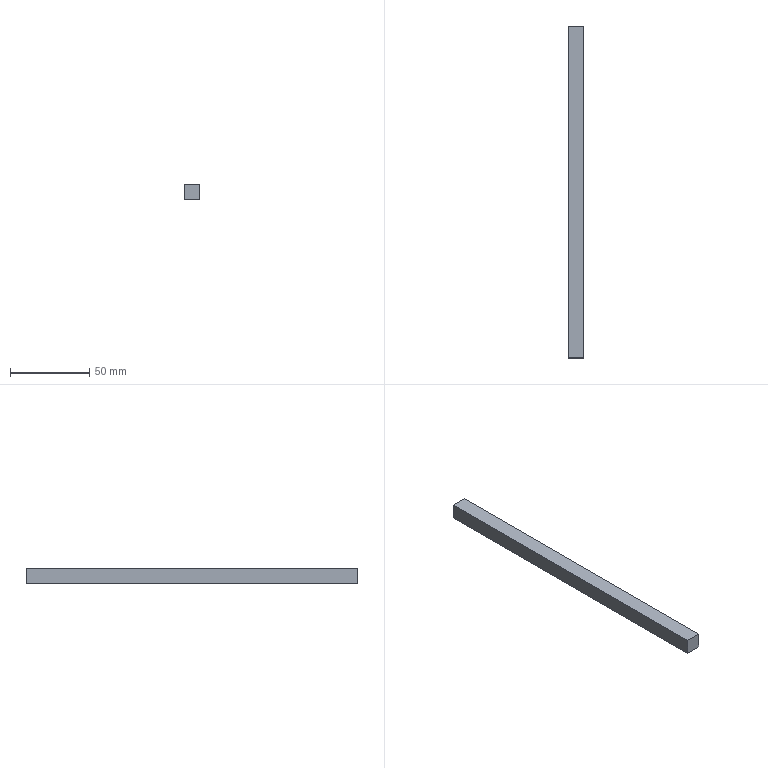Part | STEP file | 001-004-Feeding mechanism shaft entry channel baffle | 1 solid | 6 faces | box 10 x 210 x 10 mm | volume 21000 mm3 | plane 6
STEP:
#1=CARTESIAN_POINT('',(0.,0.,0.));
#2=DIRECTION('',(0.,0.,1.));
#3=DIRECTION('',(1.,0.,0.));
#4=AXIS2_PLACEMENT_3D('',#1,#2,#3);
#5=CARTESIAN_POINT('',(5.,-105.,0.));
#6=VERTEX_POINT('',#5);
#7=CARTESIAN_POINT('',(5.,105.,0.));
#8=VERTEX_POINT('',#7);
#9=CARTESIAN_POINT('',(5.,-105.,0.));
#10=DIRECTION('',(0.,1.,0.));
#11=VECTOR('',#10,1.);
#12=LINE('',#9,#11);
#13=CARTESIAN_POINT('',(5.,-105.,10.));
#14=DIRECTION('',(-1.,0.,0.));
#15=DIRECTION('',(0.,0.,1.));
#16=AXIS2_PLACEMENT_3D('',#13,#14,#15);
#17=PLANE('',#16);
#18=CARTESIAN_POINT('',(-10.,0.));
#19=DIRECTION('',(0.,1.));
#20=VECTOR('',#19,1.);
#21=LINE('',#18,#20);
#22=(GEOMETRIC_REPRESENTATION_CONTEXT(2)PARAMETRIC_REPRESENTATION_CONTEXT()REPRESENTATION_CONTEXT('',''));
#23=DEFINITIONAL_REPRESENTATION('',(#21),#22);
#24=PCURVE('',#17,#23);
#25=CARTESIAN_POINT('',(0.,0.,0.));
#26=DIRECTION('',(0.,0.,-1.));
#27=DIRECTION('',(-1.,0.,0.));
#28=AXIS2_PLACEMENT_3D('',#25,#26,#27);
#29=PLANE('',#28);
#30=CARTESIAN_POINT('',(-5.,-105.));
#31=DIRECTION('',(0.,1.));
#32=VECTOR('',#31,1.);
#33=LINE('',#30,#32);
#34=(GEOMETRIC_REPRESENTATION_CONTEXT(2)PARAMETRIC_REPRESENTATION_CONTEXT()REPRESENTATION_CONTEXT('',''));
#35=DEFINITIONAL_REPRESENTATION('',(#33),#34);
#36=PCURVE('',#29,#35);
#37=SURFACE_CURVE('',#12,(#24,#36),.PCURVE_S1.);
#38=EDGE_CURVE('',#6,#8,#37,.T.);
#39=ORIENTED_EDGE('',*,*,#38,.T.);
#40=CARTESIAN_POINT('',(5.,105.,10.));
#41=VERTEX_POINT('',#40);
#42=CARTESIAN_POINT('',(5.,105.,10.));
#43=DIRECTION('',(0.,0.,-1.));
#44=VECTOR('',#43,1.);
#45=LINE('',#42,#44);
#46=CARTESIAN_POINT('',(0.,210.));
#47=DIRECTION('',(-1.,0.));
#48=VECTOR('',#47,1.);
#49=LINE('',#46,#48);
#50=(GEOMETRIC_REPRESENTATION_CONTEXT(2)PARAMETRIC_REPRESENTATION_CONTEXT()REPRESENTATION_CONTEXT('',''));
#51=DEFINITIONAL_REPRESENTATION('',(#49),#50);
#52=PCURVE('',#17,#51);
#53=CARTESIAN_POINT('',(-5.,105.,10.));
#54=DIRECTION('',(0.,-1.,0.));
#55=DIRECTION('',(0.,0.,-1.));
#56=AXIS2_PLACEMENT_3D('',#53,#54,#55);
#57=PLANE('',#56);
#58=CARTESIAN_POINT('',(0.,10.));
#59=DIRECTION('',(1.,0.));
#60=VECTOR('',#59,1.);
#61=LINE('',#58,#60);
#62=(GEOMETRIC_REPRESENTATION_CONTEXT(2)PARAMETRIC_REPRESENTATION_CONTEXT()REPRESENTATION_CONTEXT('',''));
#63=DEFINITIONAL_REPRESENTATION('',(#61),#62);
#64=PCURVE('',#57,#63);
#65=SURFACE_CURVE('',#45,(#52,#64),.PCURVE_S1.);
#66=EDGE_CURVE('',#41,#8,#65,.T.);
#67=ORIENTED_EDGE('',*,*,#66,.F.);
#68=CARTESIAN_POINT('',(5.,-105.,10.));
#69=VERTEX_POINT('',#68);
#70=CARTESIAN_POINT('',(5.,-105.,10.));
#71=DIRECTION('',(0.,1.,0.));
#72=VECTOR('',#71,1.);
#73=LINE('',#70,#72);
#74=CARTESIAN_POINT('',(0.,0.));
#75=DIRECTION('',(0.,1.));
#76=VECTOR('',#75,1.);
#77=LINE('',#74,#76);
#78=(GEOMETRIC_REPRESENTATION_CONTEXT(2)PARAMETRIC_REPRESENTATION_CONTEXT()REPRESENTATION_CONTEXT('',''));
#79=DEFINITIONAL_REPRESENTATION('',(#77),#78);
#80=PCURVE('',#17,#79);
#81=CARTESIAN_POINT('',(0.,0.,10.));
#82=DIRECTION('',(0.,0.,-1.));
#83=DIRECTION('',(-1.,0.,0.));
#84=AXIS2_PLACEMENT_3D('',#81,#82,#83);
#85=PLANE('',#84);
#86=CARTESIAN_POINT('',(-5.,-105.));
#87=DIRECTION('',(0.,1.));
#88=VECTOR('',#87,1.);
#89=LINE('',#86,#88);
#90=(GEOMETRIC_REPRESENTATION_CONTEXT(2)PARAMETRIC_REPRESENTATION_CONTEXT()REPRESENTATION_CONTEXT('',''));
#91=DEFINITIONAL_REPRESENTATION('',(#89),#90);
#92=PCURVE('',#85,#91);
#93=SURFACE_CURVE('',#73,(#80,#92),.PCURVE_S1.);
#94=EDGE_CURVE('',#69,#41,#93,.T.);
#95=ORIENTED_EDGE('',*,*,#94,.F.);
#96=CARTESIAN_POINT('',(5.,-105.,10.));
#97=DIRECTION('',(0.,0.,-1.));
#98=VECTOR('',#97,1.);
#99=LINE('',#96,#98);
#100=CARTESIAN_POINT('',(0.,0.));
#101=DIRECTION('',(-1.,0.));
#102=VECTOR('',#101,1.);
#103=LINE('',#100,#102);
#104=(GEOMETRIC_REPRESENTATION_CONTEXT(2)PARAMETRIC_REPRESENTATION_CONTEXT()REPRESENTATION_CONTEXT('',''));
#105=DEFINITIONAL_REPRESENTATION('',(#103),#104);
#106=PCURVE('',#17,#105);
#107=CARTESIAN_POINT('',(-5.,-105.,10.));
#108=DIRECTION('',(0.,1.,0.));
#109=DIRECTION('',(0.,0.,1.));
#110=AXIS2_PLACEMENT_3D('',#107,#108,#109);
#111=PLANE('',#110);
#112=CARTESIAN_POINT('',(0.,10.));
#113=DIRECTION('',(-1.,0.));
#114=VECTOR('',#113,1.);
#115=LINE('',#112,#114);
#116=(GEOMETRIC_REPRESENTATION_CONTEXT(2)PARAMETRIC_REPRESENTATION_CONTEXT()REPRESENTATION_CONTEXT('',''));
#117=DEFINITIONAL_REPRESENTATION('',(#115),#116);
#118=PCURVE('',#111,#117);
#119=SURFACE_CURVE('',#99,(#106,#118),.PCURVE_S1.);
#120=EDGE_CURVE('',#69,#6,#119,.T.);
#121=ORIENTED_EDGE('',*,*,#120,.T.);
#122=EDGE_LOOP('',(#39,#67,#95,#121));
#123=FACE_BOUND('',#122,.T.);
#124=ADVANCED_FACE('',(#123),#17,.F.);
#125=CARTESIAN_POINT('',(-5.,105.,0.));
#126=VERTEX_POINT('',#125);
#127=CARTESIAN_POINT('',(-5.,105.,0.));
#128=DIRECTION('',(-1.,0.,0.));
#129=VECTOR('',#128,1.);
#130=LINE('',#127,#129);
#131=CARTESIAN_POINT('',(10.,0.));
#132=DIRECTION('',(0.,-1.));
#133=VECTOR('',#132,1.);
#134=LINE('',#131,#133);
#135=(GEOMETRIC_REPRESENTATION_CONTEXT(2)PARAMETRIC_REPRESENTATION_CONTEXT()REPRESENTATION_CONTEXT('',''));
#136=DEFINITIONAL_REPRESENTATION('',(#134),#135);
#137=PCURVE('',#57,#136);
#138=CARTESIAN_POINT('',(5.,105.));
#139=DIRECTION('',(1.,0.));
#140=VECTOR('',#139,1.);
#141=LINE('',#138,#140);
#142=(GEOMETRIC_REPRESENTATION_CONTEXT(2)PARAMETRIC_REPRESENTATION_CONTEXT()REPRESENTATION_CONTEXT('',''));
#143=DEFINITIONAL_REPRESENTATION('',(#141),#142);
#144=PCURVE('',#29,#143);
#145=SURFACE_CURVE('',#130,(#137,#144),.PCURVE_S1.);
#146=EDGE_CURVE('',#8,#126,#145,.T.);
#147=ORIENTED_EDGE('',*,*,#146,.T.);
#148=CARTESIAN_POINT('',(-5.,105.,10.));
#149=VERTEX_POINT('',#148);
#150=CARTESIAN_POINT('',(-5.,105.,10.));
#151=DIRECTION('',(0.,0.,-1.));
#152=VECTOR('',#151,1.);
#153=LINE('',#150,#152);
#154=CARTESIAN_POINT('',(0.,0.));
#155=DIRECTION('',(1.,0.));
#156=VECTOR('',#155,1.);
#157=LINE('',#154,#156);
#158=(GEOMETRIC_REPRESENTATION_CONTEXT(2)PARAMETRIC_REPRESENTATION_CONTEXT()REPRESENTATION_CONTEXT('',''));
#159=DEFINITIONAL_REPRESENTATION('',(#157),#158);
#160=PCURVE('',#57,#159);
#161=CARTESIAN_POINT('',(-5.,-105.,10.));
#162=DIRECTION('',(1.,0.,0.));
#163=DIRECTION('',(0.,0.,-1.));
#164=AXIS2_PLACEMENT_3D('',#161,#162,#163);
#165=PLANE('',#164);
#166=CARTESIAN_POINT('',(0.,210.));
#167=DIRECTION('',(1.,0.));
#168=VECTOR('',#167,1.);
#169=LINE('',#166,#168);
#170=(GEOMETRIC_REPRESENTATION_CONTEXT(2)PARAMETRIC_REPRESENTATION_CONTEXT()REPRESENTATION_CONTEXT('',''));
#171=DEFINITIONAL_REPRESENTATION('',(#169),#170);
#172=PCURVE('',#165,#171);
#173=SURFACE_CURVE('',#153,(#160,#172),.PCURVE_S1.);
#174=EDGE_CURVE('',#149,#126,#173,.T.);
#175=ORIENTED_EDGE('',*,*,#174,.F.);
#176=CARTESIAN_POINT('',(-5.,105.,10.));
#177=DIRECTION('',(-1.,0.,0.));
#178=VECTOR('',#177,1.);
#179=LINE('',#176,#178);
#180=CARTESIAN_POINT('',(0.,0.));
#181=DIRECTION('',(0.,-1.));
#182=VECTOR('',#181,1.);
#183=LINE('',#180,#182);
#184=(GEOMETRIC_REPRESENTATION_CONTEXT(2)PARAMETRIC_REPRESENTATION_CONTEXT()REPRESENTATION_CONTEXT('',''));
#185=DEFINITIONAL_REPRESENTATION('',(#183),#184);
#186=PCURVE('',#57,#185);
#187=CARTESIAN_POINT('',(5.,105.));
#188=DIRECTION('',(1.,0.));
#189=VECTOR('',#188,1.);
#190=LINE('',#187,#189);
#191=(GEOMETRIC_REPRESENTATION_CONTEXT(2)PARAMETRIC_REPRESENTATION_CONTEXT()REPRESENTATION_CONTEXT('',''));
#192=DEFINITIONAL_REPRESENTATION('',(#190),#191);
#193=PCURVE('',#85,#192);
#194=SURFACE_CURVE('',#179,(#186,#193),.PCURVE_S1.);
#195=EDGE_CURVE('',#41,#149,#194,.T.);
#196=ORIENTED_EDGE('',*,*,#195,.F.);
#197=ORIENTED_EDGE('',*,*,#66,.T.);
#198=EDGE_LOOP('',(#147,#175,#196,#197));
#199=FACE_BOUND('',#198,.T.);
#200=ADVANCED_FACE('',(#199),#57,.F.);
#201=CARTESIAN_POINT('',(-5.,-105.,0.));
#202=VERTEX_POINT('',#201);
#203=CARTESIAN_POINT('',(-5.,-105.,0.));
#204=DIRECTION('',(0.,-1.,0.));
#205=VECTOR('',#204,1.);
#206=LINE('',#203,#205);
#207=CARTESIAN_POINT('',(10.,0.));
#208=DIRECTION('',(0.,-1.));
#209=VECTOR('',#208,1.);
#210=LINE('',#207,#209);
#211=(GEOMETRIC_REPRESENTATION_CONTEXT(2)PARAMETRIC_REPRESENTATION_CONTEXT()REPRESENTATION_CONTEXT('',''));
#212=DEFINITIONAL_REPRESENTATION('',(#210),#211);
#213=PCURVE('',#165,#212);
#214=CARTESIAN_POINT('',(5.,-105.));
#215=DIRECTION('',(0.,-1.));
#216=VECTOR('',#215,1.);
#217=LINE('',#214,#216);
#218=(GEOMETRIC_REPRESENTATION_CONTEXT(2)PARAMETRIC_REPRESENTATION_CONTEXT()REPRESENTATION_CONTEXT('',''));
#219=DEFINITIONAL_REPRESENTATION('',(#217),#218);
#220=PCURVE('',#29,#219);
#221=SURFACE_CURVE('',#206,(#213,#220),.PCURVE_S1.);
#222=EDGE_CURVE('',#126,#202,#221,.T.);
#223=ORIENTED_EDGE('',*,*,#222,.T.);
#224=CARTESIAN_POINT('',(-5.,-105.,10.));
#225=VERTEX_POINT('',#224);
#226=CARTESIAN_POINT('',(-5.,-105.,10.));
#227=DIRECTION('',(0.,0.,-1.));
#228=VECTOR('',#227,1.);
#229=LINE('',#226,#228);
#230=CARTESIAN_POINT('',(0.,0.));
#231=DIRECTION('',(1.,0.));
#232=VECTOR('',#231,1.);
#233=LINE('',#230,#232);
#234=(GEOMETRIC_REPRESENTATION_CONTEXT(2)PARAMETRIC_REPRESENTATION_CONTEXT()REPRESENTATION_CONTEXT('',''));
#235=DEFINITIONAL_REPRESENTATION('',(#233),#234);
#236=PCURVE('',#165,#235);
#237=CARTESIAN_POINT('',(0.,0.));
#238=DIRECTION('',(-1.,0.));
#239=VECTOR('',#238,1.);
#240=LINE('',#237,#239);
#241=(GEOMETRIC_REPRESENTATION_CONTEXT(2)PARAMETRIC_REPRESENTATION_CONTEXT()REPRESENTATION_CONTEXT('',''));
#242=DEFINITIONAL_REPRESENTATION('',(#240),#241);
#243=PCURVE('',#111,#242);
#244=SURFACE_CURVE('',#229,(#236,#243),.PCURVE_S1.);
#245=EDGE_CURVE('',#225,#202,#244,.T.);
#246=ORIENTED_EDGE('',*,*,#245,.F.);
#247=CARTESIAN_POINT('',(-5.,-105.,10.));
#248=DIRECTION('',(0.,-1.,0.));
#249=VECTOR('',#248,1.);
#250=LINE('',#247,#249);
#251=CARTESIAN_POINT('',(0.,0.));
#252=DIRECTION('',(0.,-1.));
#253=VECTOR('',#252,1.);
#254=LINE('',#251,#253);
#255=(GEOMETRIC_REPRESENTATION_CONTEXT(2)PARAMETRIC_REPRESENTATION_CONTEXT()REPRESENTATION_CONTEXT('',''));
#256=DEFINITIONAL_REPRESENTATION('',(#254),#255);
#257=PCURVE('',#165,#256);
#258=CARTESIAN_POINT('',(5.,-105.));
#259=DIRECTION('',(0.,-1.));
#260=VECTOR('',#259,1.);
#261=LINE('',#258,#260);
#262=(GEOMETRIC_REPRESENTATION_CONTEXT(2)PARAMETRIC_REPRESENTATION_CONTEXT()REPRESENTATION_CONTEXT('',''));
#263=DEFINITIONAL_REPRESENTATION('',(#261),#262);
#264=PCURVE('',#85,#263);
#265=SURFACE_CURVE('',#250,(#257,#264),.PCURVE_S1.);
#266=EDGE_CURVE('',#149,#225,#265,.T.);
#267=ORIENTED_EDGE('',*,*,#266,.F.);
#268=ORIENTED_EDGE('',*,*,#174,.T.);
#269=EDGE_LOOP('',(#223,#246,#267,#268));
#270=FACE_BOUND('',#269,.T.);
#271=ADVANCED_FACE('',(#270),#165,.F.);
#272=CARTESIAN_POINT('',(-5.,-105.,0.));
#273=DIRECTION('',(1.,0.,0.));
#274=VECTOR('',#273,1.);
#275=LINE('',#272,#274);
#276=CARTESIAN_POINT('',(-10.,0.));
#277=DIRECTION('',(0.,1.));
#278=VECTOR('',#277,1.);
#279=LINE('',#276,#278);
#280=(GEOMETRIC_REPRESENTATION_CONTEXT(2)PARAMETRIC_REPRESENTATION_CONTEXT()REPRESENTATION_CONTEXT('',''));
#281=DEFINITIONAL_REPRESENTATION('',(#279),#280);
#282=PCURVE('',#111,#281);
#283=CARTESIAN_POINT('',(5.,-105.));
#284=DIRECTION('',(-1.,0.));
#285=VECTOR('',#284,1.);
#286=LINE('',#283,#285);
#287=(GEOMETRIC_REPRESENTATION_CONTEXT(2)PARAMETRIC_REPRESENTATION_CONTEXT()REPRESENTATION_CONTEXT('',''));
#288=DEFINITIONAL_REPRESENTATION('',(#286),#287);
#289=PCURVE('',#29,#288);
#290=SURFACE_CURVE('',#275,(#282,#289),.PCURVE_S1.);
#291=EDGE_CURVE('',#202,#6,#290,.T.);
#292=ORIENTED_EDGE('',*,*,#291,.T.);
#293=ORIENTED_EDGE('',*,*,#120,.F.);
#294=CARTESIAN_POINT('',(-5.,-105.,10.));
#295=DIRECTION('',(1.,0.,0.));
#296=VECTOR('',#295,1.);
#297=LINE('',#294,#296);
#298=CARTESIAN_POINT('',(0.,0.));
#299=DIRECTION('',(0.,1.));
#300=VECTOR('',#299,1.);
#301=LINE('',#298,#300);
#302=(GEOMETRIC_REPRESENTATION_CONTEXT(2)PARAMETRIC_REPRESENTATION_CONTEXT()REPRESENTATION_CONTEXT('',''));
#303=DEFINITIONAL_REPRESENTATION('',(#301),#302);
#304=PCURVE('',#111,#303);
#305=CARTESIAN_POINT('',(5.,-105.));
#306=DIRECTION('',(-1.,0.));
#307=VECTOR('',#306,1.);
#308=LINE('',#305,#307);
#309=(GEOMETRIC_REPRESENTATION_CONTEXT(2)PARAMETRIC_REPRESENTATION_CONTEXT()REPRESENTATION_CONTEXT('',''));
#310=DEFINITIONAL_REPRESENTATION('',(#308),#309);
#311=PCURVE('',#85,#310);
#312=SURFACE_CURVE('',#297,(#304,#311),.PCURVE_S1.);
#313=EDGE_CURVE('',#225,#69,#312,.T.);
#314=ORIENTED_EDGE('',*,*,#313,.F.);
#315=ORIENTED_EDGE('',*,*,#245,.T.);
#316=EDGE_LOOP('',(#292,#293,#314,#315));
#317=FACE_BOUND('',#316,.T.);
#318=ADVANCED_FACE('',(#317),#111,.F.);
#319=ORIENTED_EDGE('',*,*,#94,.T.);
#320=ORIENTED_EDGE('',*,*,#195,.T.);
#321=ORIENTED_EDGE('',*,*,#266,.T.);
#322=ORIENTED_EDGE('',*,*,#313,.T.);
#323=EDGE_LOOP('',(#319,#320,#321,#322));
#324=FACE_BOUND('',#323,.T.);
#325=ADVANCED_FACE('',(#324),#85,.F.);
#326=ORIENTED_EDGE('',*,*,#38,.F.);
#327=ORIENTED_EDGE('',*,*,#291,.F.);
#328=ORIENTED_EDGE('',*,*,#222,.F.);
#329=ORIENTED_EDGE('',*,*,#146,.F.);
#330=EDGE_LOOP('',(#326,#327,#328,#329));
#331=FACE_BOUND('',#330,.T.);
#332=ADVANCED_FACE('',(#331),#29,.T.);
#333=CLOSED_SHELL('',(#124,#200,#271,#318,#325,#332));
#334=MANIFOLD_SOLID_BREP('',#333);
#335=(LENGTH_UNIT()NAMED_UNIT(*)SI_UNIT(.MILLI.,.METRE.));
#336=UNCERTAINTY_MEASURE_WITH_UNIT(LENGTH_MEASURE(0.0000001),#335,'','');
#337=(NAMED_UNIT(*)PLANE_ANGLE_UNIT()SI_UNIT($,.RADIAN.));
#338=(NAMED_UNIT(*)SI_UNIT($,.STERADIAN.)SOLID_ANGLE_UNIT());
#339=(GEOMETRIC_REPRESENTATION_CONTEXT(3)GLOBAL_UNCERTAINTY_ASSIGNED_CONTEXT((#336))GLOBAL_UNIT_ASSIGNED_CONTEXT((#335,#337,#338))REPRESENTATION_CONTEXT('',''));
#340=ADVANCED_BREP_SHAPE_REPRESENTATION('',(#4,#334),#339);